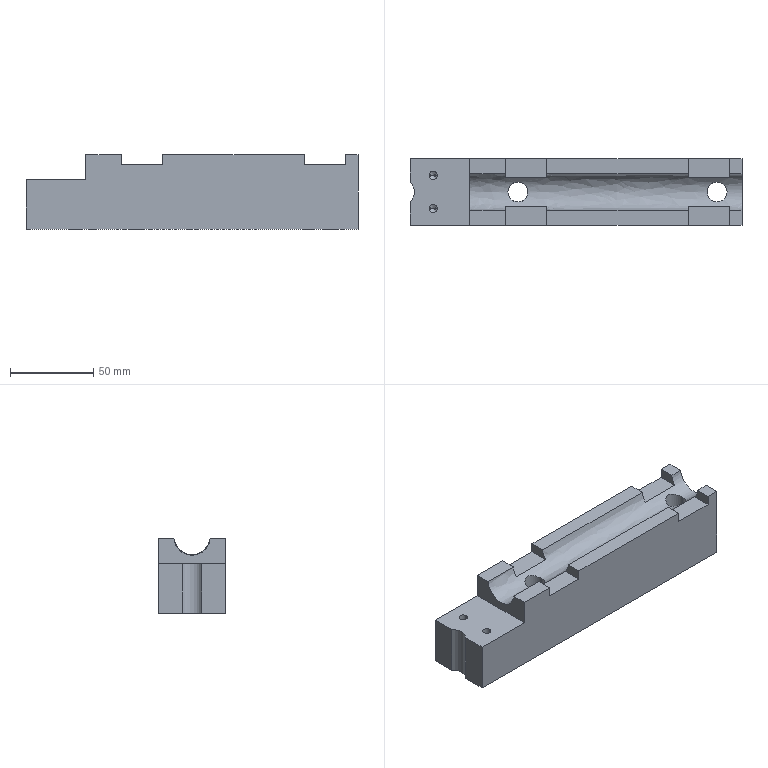NC program | NX | posted with a generic post
Lines 3384 to 4303 of 104568:
(FLOOR_WALL_1 , TOOL : D6)
N6760 T06 M6
N6762 G54
N6764 G17 G0 G90 X71.103 Y-24.5 S9500 M3
N6766 G43 Z30. H6
N6768 Z-4.5
N6770 G94 G1 Z-6. F1250.
N6772 Y-22.48
N6774 G3 X70.803 Y-23. R0.6
N6776 G1 Y-5.535
N6778 X73.431 Y-5.537
N6780 Y-23.
N6782 X76.059
N6784 Y-5.538
N6786 X78.687 Y-5.54
N6788 Y-23.
N6790 X81.316
N6792 Y-5.542
N6794 X83.944 Y-5.543
N6796 Y-23.
N6798 X86.572
N6800 Y-5.545
N6802 X89.2 Y-5.546
N6804 Y-23.
N6806 G2 X88.9 Y-23.52 R0.6
N6808 G1 X87.202 Y-24.5
N6810 Z-4.5
N6812 G0 Z30.
N6814 X87.502
N6816 Z-4.5
N6818 G1 Z-6.
N6820 X89.2 Y-23.52
N6822 G3 X89.5 Y-23. R0.6
N6824 G1 Y-5.546
N6826 G3 X89.2 Y-5.027 R0.6
N6828 G1 X87.5 Y-4.045
N6830 Z-4.5
N6832 G0 Z30.
N6834 X72.496 Y-4.036
N6836 Z-4.5
N6838 G1 Z-6.
N6840 X70.8 Y-5.015
N6842 G3 X70.5 Y-5.535 R0.6
N6844 G1 Y-23.
N6846 G3 X70.8 Y-23.52 R0.6
N6848 G1 X72.498 Y-24.5
N6850 Z-4.5
N6852 G0 Z30.
N6854 X71.101 Y3.926
N6856 Z-4.5
N6858 G1 Z-6.
N6860 X71.103 Y5.946
N6862 G3 X70.803 Y5.427 R0.6
N6864 G1 Y23.
N6866 X73.431
N6868 Y5.426
N6870 X76.059 Y5.425
N6872 Y23.
N6874 X78.687
N6876 Y5.425
N6878 X81.316 Y5.424
N6880 Y23.
N6882 X83.944
N6884 Y5.424
N6886 X86.572 Y5.423
N6888 Y23.
N6890 X89.2
N6892 Y5.422
N6894 G2 X88.9 Y4.902 R0.6
N6896 G1 X87.203 Y3.922
N6898 Z-4.5
N6900 G0 Z30.
N6902 X87.503
N6904 Z-4.5
N6906 G1 Z-6.
N6908 X89.2 Y4.902
N6910 G3 X89.5 Y5.422 R0.6
N6912 G1 Y23.
N6914 G3 X89.2 Y23.52 R0.6
N6916 G1 X87.502 Y24.5
N6918 Z-4.5
N6920 G0 Z30.
N6922 X72.498
N6924 Z-4.5
N6926 G1 Z-6.
N6928 X70.8 Y23.52
N6930 G3 X70.5 Y23. R0.6
N6932 G1 Y5.427
N6934 G3 X70.8 Y4.907 R0.6
N6936 G1 X72.499 Y3.926
N6938 Z-4.5
N6940 G0 Z30.
N6942 X-38.899 Y3.981
N6944 Z-4.5
N6946 G1 Z-6.
N6948 X-38.897 Y6.001
N6950 G3 X-39.197 Y5.481 R0.6
N6952 G1 Y23.
N6954 X-36.569
N6956 Y5.48
N6958 X-33.941
N6960 Y23.
N6962 X-31.313
N6964 Y5.479
N6966 X-28.684
N6968 Y23.
N6970 X-26.056
N6972 Y5.479
N6974 X-23.428
N6976 Y23.
N6978 X-20.8
N6980 Y5.479
N6982 G2 X-21.1 Y4.96 R0.6
N6984 G1 X-22.798 Y3.979
N6986 Z-4.5
N6988 G0 Z30.
N6990 X-22.498
N6992 Z-4.5
N6994 G1 Z-6.
N6996 X-20.8 Y4.96
N6998 G3 X-20.5 Y5.479 R0.6
N7000 G1 Y23.
N7002 G3 X-20.8 Y23.52 R0.6
N7004 G1 X-22.498 Y24.5
N7006 Z-4.5
N7008 G0 Z30.
N7010 X-37.502
N7012 Z-4.5
N7014 G1 Z-6.
N7016 X-39.2 Y23.52
N7018 G3 X-39.5 Y23. R0.6
N7020 G1 Y5.481
N7022 G3 X-39.2 Y4.962 R0.6
N7024 G1 X-37.499 Y3.98
N7026 Z-4.5
N7028 G0 Z30.
N7030 X-38.897 Y-24.5
N7032 Z-4.5
N7034 G1 Z-6.
N7036 Y-22.48
N7038 G3 X-39.197 Y-23. R0.6
N7040 G1 Y-5.482
N7042 X-36.569 Y-5.484
N7044 Y-23.
N7046 X-33.941
N7048 Y-5.485
N7050 X-31.313 Y-5.486
N7052 Y-23.
N7054 X-28.684
N7056 Y-5.488
N7058 X-26.056 Y-5.491
N7060 Y-23.
N7062 X-23.428
N7064 Y-5.493
N7066 X-20.8 Y-5.496
N7068 Y-23.
N7070 G2 X-21.1 Y-23.52 R0.6
N7072 G1 X-22.798 Y-24.5
N7074 Z-4.5
N7076 G0 Z30.
N7078 X-22.498
N7080 Z-4.5
N7082 G1 Z-6.
N7084 X-20.8 Y-23.52
N7086 G3 X-20.5 Y-23. R0.6
N7088 G1 Y-5.496
N7090 G3 X-20.8 Y-4.977 R0.6
N7092 G1 X-22.501 Y-3.994
N7094 Z-4.5
N7096 G0 Z30.
N7098 X-37.504 Y-3.983
N7100 Z-4.5
N7102 G1 Z-6.
N7104 X-39.2 Y-4.963
N7106 G3 X-39.5 Y-5.482 R0.6
N7108 G1 Y-23.
N7110 G3 X-39.2 Y-23.52 R0.6
N7112 G1 X-37.502 Y-24.5
N7114 Z-4.5
N7116 G0 Z30.
N7118 X-104.123 Y-23.995
N7120 Z-13.5
N7122 G1 Z-15.
N7124 X-103.3 Y-23.52
N7126 G3 X-103. Y-23. R0.6
N7128 G1 Y23.
N7130 X-100.025
N7132 Y-23.
N7134 X-97.05
N7136 Y23.
N7138 X-94.075
N7140 Y-23.
N7142 X-91.1
N7144 Y23.
N7146 X-88.125
N7148 Y-23.
N7150 X-85.15
N7152 Y23.
N7154 X-82.175
N7156 Y-23.
N7158 X-79.2
N7160 Y23.
N7162 X-76.225
N7164 Y-23.
N7166 X-73.25
N7168 Y23.
N7170 X-70.275
N7172 Y-23.
N7174 X-67.3
N7176 Y23.
N7178 G3 X-67.6 Y23.52 R0.6
N7180 G1 X-69.298 Y24.5
N7182 Z-13.5
N7184 G0 Z30.
N7186 X-68.998 Y-24.5
N7188 Z-13.5
N7190 G1 Z-15.
N7192 X-67.3 Y-23.52
N7194 G3 X-67. Y-23. R0.6
N7196 G1 Y23.
N7198 G3 X-67.3 Y23.52 R0.6
N7200 G1 X-68.998 Y24.5
N7202 Z-13.5
N7204 G0 Z30.
(FIXED_CONTOUR , TOOL : D6)
N7206 X-64.628 Y6.929
N7208 Z3.6
N7210 G1 Z-1.91 F500.
N7212 G2 X-64.472 Y7.508 R0.6
N7214 G1 X-64.378 Y7.602 Z-1.535 F2500.
N7216 X-64.225 Y7.755 Z-0.73
N7218 X-64.2 Y7.78 Z-0.573
N7220 X-64.091 Y7.889 Z0.362
N7222 X-63.94 Z0.366
N7224 X-64.047 Y7.781 Z-0.559
N7226 X-64.089 Y7.74 Z-0.823
N7228 X-64.21 Y7.619 Z-1.458
N7230 X-64.256 Y7.573 Z-1.656
N7232 X-64.414 Y7.415 Z-2.238
N7234 X-64.479 Y7.35 Z-2.423
N7236 X-64.488 Y7.159 Z-2.949
N7238 X-64.259 Y7.387 Z-2.324
N7240 X-64.215 Y7.431 Z-2.186
N7242 X-64.097 Y7.549 Z-1.749
N7244 X-64.007 Y7.639 Z-1.365
N7246 X-63.926 Y7.721 Z-0.934
N7248 X-63.864 Y7.783 Z-0.542
N7250 X-63.758 Y7.889 Z0.37
N7252 X-63.553 Z0.375
N7254 X-63.657 Y7.784 Z-0.523
N7256 X-63.742 Y7.7 Z-1.059
N7258 X-63.78 Y7.661 Z-1.26
N7260 X-63.919 Y7.523 Z-1.853
N7262 X-63.996 Y7.446 Z-2.139
N7264 X-64.085 Y7.356 Z-2.42
N7266 X-64.385 Y7.057 Z-3.23
N7268 X-64.493 Y6.948 Z-3.46
N7270 X-64.498 Y6.72 Z-3.942
N7272 X-64.161 Y7.057 Z-3.231
N7274 X-64.075 Y7.143 Z-3.01
N7276 X-63.896 Y7.322 Z-2.525
N7278 X-63.757 Y7.461 Z-2.088
N7280 X-63.724 Y7.494 Z-1.966
N7282 X-63.537 Y7.681 Z-1.169
N7284 X-63.433 Y7.785 Z-0.507
N7286 X-63.329 Y7.888 Z0.38
N7288 X-63.081 Z0.386
N7290 X-63.185 Y7.785 Z-0.491
N7292 X-63.289 Y7.681 Z-1.17
N7294 X-63.497 Y7.473 Z-2.051
N7296 X-63.686 Y7.284 Z-2.642
N7298 X-63.913 Y7.057 Z-3.232
N7300 X-64.33 Y6.64 Z-4.104
N7302 X-64.5 Y6.47 Z-4.396
N7304 X-64.501 Y6.209 Z-4.83
N7306 X-64.071 Y6.64 Z-4.104
N7308 X-63.654 Y7.057 Z-3.233
N7310 X-63.446 Y7.265 Z-2.701
N7312 X-63.238 Y7.473 Z-2.054
N7314 X-63.03 Y7.681 Z-1.172
N7316 X-62.926 Y7.785 Z-0.475
N7318 X-62.822 Y7.888 Z0.392
N7320 X-62.556 Z0.399
N7322 X-62.66 Y7.784 Z-0.465
N7324 X-62.764 Y7.681 Z-1.174
N7326 X-62.972 Y7.473 Z-2.056
N7328 X-63.18 Y7.265 Z-2.702
N7330 X-63.388 Y7.057 Z-3.234
N7332 X-63.804 Y6.64 Z-4.104
N7334 X-64.221 Y6.223 Z-4.81
N7336 X-64.5 Y5.944 Z-5.23
N7338 Y5.738 Z-5.522
N7340 Y5.655 Z-5.629
N7342 X-64.35 Y5.806 Z-5.43
N7344 X-63.933 Y6.223 Z-4.81
N7346 X-63.516 Y6.64 Z-4.104
N7348 X-63.099 Y7.057 Z-3.235
N7350 X-62.891 Y7.265 Z-2.703
N7352 X-62.683 Y7.473 Z-2.059
N7354 X-62.475 Y7.681 Z-1.174
N7356 X-62.371 Y7.784 Z-0.471
N7358 X-62.267 Y7.888 Z0.406
N7360 X-61.967 Z0.413
N7362 X-62.071 Y7.784 Z-0.478
N7364 X-62.175 Y7.681 Z-1.174
N7366 X-62.383 Y7.473 Z-2.059
N7368 X-62.591 Y7.265 Z-2.703
N7370 X-62.799 Y7.057 Z-3.235
N7372 X-63.215 Y6.64 Z-4.103
N7374 X-63.632 Y6.223 Z-4.81
N7376 X-64.049 Y5.806 Z-5.43
N7378 X-64.5 Y5.355 Z-6.009
N7380 Y5.054 Z-6.354
N7382 X-64.165 Y5.389 Z-5.971
N7384 X-63.748 Y5.806 Z-5.43
N7386 X-63.331 Y6.223 Z-4.81
N7388 X-62.914 Y6.64 Z-4.102
N7390 X-62.497 Y7.057 Z-3.236
N7392 X-62.289 Y7.265 Z-2.704
N7394 X-62.081 Y7.473 Z-2.06
N7396 X-61.873 Y7.681 Z-1.175
N7398 X-61.769 Y7.784 Z-0.485
N7400 X-61.665 Y7.889 Z0.419
N7402 X-61.364 Z0.424
N7404 X-61.468 Y7.784 Z-0.492
N7406 X-61.572 Y7.681 Z-1.172
N7408 X-61.78 Y7.473 Z-2.06
N7410 X-61.988 Y7.265 Z-2.705
N7412 X-62.196 Y7.057 Z-3.237
N7414 X-62.613 Y6.64 Z-4.101
N7416 X-63.03 Y6.223 Z-4.81
N7418 X-63.447 Y5.806 Z-5.429
N7420 X-63.864 Y5.389 Z-5.972
N7422 X-64.28 Y4.972 Z-6.443
N7424 X-64.5 Y4.753 Z-6.666
N7426 Y4.555 Z-6.862
N7428 Y4.451 Z-6.952
N7430 X-64.396 Y4.555 Z-6.862
N7432 X-63.979 Y4.972 Z-6.443
N7434 X-63.562 Y5.389 Z-5.972
N7436 X-63.145 Y5.806 Z-5.428
N7438 X-62.729 Y6.223 Z-4.809
N7440 X-62.312 Y6.64 Z-4.1
N7442 X-61.895 Y7.057 Z-3.237
N7444 X-61.687 Y7.265 Z-2.706
N7446 X-61.479 Y7.473 Z-2.06
N7448 X-61.271 Y7.681 Z-1.169
N7450 X-61.167 Y7.784 Z-0.499
N7452 X-61.063 Y7.889 Z0.43
N7454 X-60.761 Z0.435
N7456 X-60.866 Y7.784 Z-0.504
N7458 X-60.97 Y7.681 Z-1.167
N7460 X-61.178 Y7.473 Z-2.061
N7462 X-61.386 Y7.265 Z-2.706
N7464 X-61.593 Y7.057 Z-3.238
N7466 X-62.01 Y6.64 Z-4.099
N7468 X-62.427 Y6.223 Z-4.809
N7470 X-62.844 Y5.806 Z-5.427
N7472 X-63.261 Y5.389 Z-5.972
N7474 X-63.678 Y4.972 Z-6.443
N7476 X-64.095 Y4.555 Z-6.862
N7478 X-64.5 Y4.15 Z-7.214
N7480 X-64.501 Y3.848 Z-7.475
N7482 X-63.793 Y4.555 Z-6.862
N7484 X-63.377 Y4.972 Z-6.444
N7486 X-62.96 Y5.389 Z-5.971
N7488 X-62.543 Y5.806 Z-5.427
N7490 X-62.126 Y6.223 Z-4.808
N7492 X-61.709 Y6.64 Z-4.099
N7494 X-61.292 Y7.057 Z-3.238
N7496 X-61.084 Y7.265 Z-2.707
N7498 X-60.876 Y7.473 Z-2.061
N7500 X-60.668 Y7.681 Z-1.166
N7502 X-60.564 Y7.784 Z-0.509
N7504 X-60.46 Y7.889 Z0.44
N7506 X-60.159 Z0.445
N7508 X-60.263 Y7.784 Z-0.513
N7510 X-60.367 Y7.681 Z-1.164
N7512 X-60.575 Y7.473 Z-2.061
N7514 X-60.783 Y7.265 Z-2.708
N7516 X-60.991 Y7.057 Z-3.238
N7518 X-61.408 Y6.64 Z-4.098
N7520 X-61.824 Y6.223 Z-4.807
N7522 X-62.241 Y5.806 Z-5.426
N7524 X-62.658 Y5.389 Z-5.971
N7526 X-63.075 Y4.972 Z-6.444
N7528 X-63.492 Y4.555 Z-6.863
N7530 X-64.326 Y3.722 Z-7.586
N7532 X-64.501 Y3.547 Z-7.71
N7534 Y3.247 Z-7.923
N7536 X-64.026 Y3.722 Z-7.586
N7538 X-63.192 Y4.555 Z-6.862
N7540 X-62.775 Y4.972 Z-6.444
N7542 X-62.358 Y5.389 Z-5.97
N7544 X-61.941 Y5.806 Z-5.425
N7546 X-61.524 Y6.223 Z-4.805
N7548 X-61.107 Y6.64 Z-4.097
N7550 X-60.691 Y7.057 Z-3.236
N7552 X-60.483 Y7.265 Z-2.708
N7554 X-60.275 Y7.473 Z-2.062
N7556 X-60.067 Y7.68 Z-1.165
N7558 X-59.963 Y7.784 Z-0.515
N7560 X-59.859 Y7.889 Z0.449
N7562 X-59.557 Y7.888 Z0.452
N7564 X-59.661 Y7.784 Z-0.517
N7566 X-59.765 Y7.68 Z-1.17
N7568 X-59.973 Y7.473 Z-2.063
N7570 X-60.181 Y7.265 Z-2.709
N7572 X-60.389 Y7.057 Z-3.235
N7574 X-60.806 Y6.64 Z-4.095
N7576 X-61.223 Y6.223 Z-4.803
N7578 X-61.64 Y5.806 Z-5.424
N7580 X-62.056 Y5.389 Z-5.969
N7582 X-62.473 Y4.972 Z-6.444
N7584 X-62.89 Y4.555 Z-6.862
N7586 X-63.724 Y3.722 Z-7.586
N7588 X-64.501 Y2.945 Z-8.137
N7590 Y2.888 Z-8.178
N7592 Y2.643 Z-8.321
N7594 X-64.256 Y2.888 Z-8.178
N7596 X-63.422 Y3.722 Z-7.586
N7598 X-62.589 Y4.555 Z-6.861
N7600 X-62.172 Y4.972 Z-6.443
N7602 X-61.755 Y5.389 Z-5.968
N7604 X-61.338 Y5.806 Z-5.423
N7606 X-60.921 Y6.223 Z-4.801
N7608 X-60.504 Y6.64 Z-4.094
N7610 X-60.087 Y7.057 Z-3.233
N7612 X-59.879 Y7.265 Z-2.709
N7614 X-59.671 Y7.472 Z-2.064
N7616 X-59.464 Y7.68 Z-1.174
N7618 X-59.36 Y7.784 Z-0.518
N7620 X-59.256 Y7.888 Z0.455
N7622 X-58.954 Z0.458
N7624 X-59.058 Y7.784 Z-0.52
N7626 X-59.162 Y7.68 Z-1.177
N7628 X-59.37 Y7.472 Z-2.066
N7630 X-59.578 Y7.265 Z-2.71
N7632 X-59.785 Y7.057 Z-3.232
N7634 X-60.202 Y6.64 Z-4.093
N7636 X-60.619 Y6.223 Z-4.8
N7638 X-61.036 Y5.806 Z-5.422
N7640 X-61.453 Y5.389 Z-5.967
N7642 X-61.87 Y4.972 Z-6.443
N7644 X-62.287 Y4.555 Z-6.857
N7646 X-63.121 Y3.722 Z-7.586
N7648 X-63.954 Y2.888 Z-8.179
N7650 X-64.501 Y2.341 Z-8.497
N7652 Y2.04 Z-8.672
N7654 X-63.653 Y2.888 Z-8.179
N7656 X-62.819 Y3.722 Z-7.585
N7658 X-61.985 Y4.555 Z-6.854
N7660 X-61.568 Y4.972 Z-6.442
N7662 X-61.151 Y5.389 Z-5.967
N7664 X-60.734 Y5.806 Z-5.422
N7666 X-60.318 Y6.223 Z-4.8
N7668 X-59.901 Y6.64 Z-4.094
N7670 X-59.484 Y7.057 Z-3.23
N7672 X-59.276 Y7.265 Z-2.71
N7674 X-59.068 Y7.472 Z-2.068
N7676 X-58.861 Y7.68 Z-1.179
N7678 X-58.757 Y7.784 Z-0.522
N7680 X-58.653 Y7.888 Z0.461
N7682 X-58.351 Y7.887 Z0.464
N7684 X-58.455 Y7.783 Z-0.523
N7686 X-58.559 Y7.68 Z-1.181
N7688 X-58.767 Y7.472 Z-2.07
N7690 X-58.974 Y7.264 Z-2.711
N7692 X-59.182 Y7.057 Z-3.228
N7694 X-59.599 Y6.64 Z-4.095
N7696 X-60.016 Y6.223 Z-4.8
N7698 X-60.433 Y5.806 Z-5.422
N7700 X-60.85 Y5.389 Z-5.966
N7702 X-61.266 Y4.972 Z-6.442
N7704 X-61.683 Y4.555 Z-6.852
N7706 X-62.517 Y3.722 Z-7.585
N7708 X-63.351 Y2.888 Z-8.179
N7710 X-64.185 Y2.054 Z-8.666
N7712 X-64.501 Y1.738 Z-8.814
N7714 Y1.436 Z-8.955
N7716 X-63.883 Y2.054 Z-8.666
N7718 X-63.049 Y2.888 Z-8.179
N7720 X-62.215 Y3.722 Z-7.585
N7722 X-61.382 Y4.555 Z-6.852
N7724 X-60.965 Y4.972 Z-6.441
N7726 X-60.548 Y5.389 Z-5.966
N7728 X-60.131 Y5.806 Z-5.422
N7730 X-59.714 Y6.223 Z-4.801
N7732 X-59.297 Y6.64 Z-4.096
N7734 X-58.88 Y7.057 Z-3.226
N7736 X-58.673 Y7.264 Z-2.711
N7738 X-58.465 Y7.472 Z-2.071
N7740 X-58.257 Y7.68 Z-1.181
N7742 X-58.154 Y7.783 Z-0.522
N7744 X-58.05 Y7.887 Z0.467
N7746 X-57.748 Z0.47
N7748 X-57.852 Y7.783 Z-0.522
N7750 X-57.956 Y7.68 Z-1.181
N7752 X-58.163 Y7.472 Z-2.072
N7754 X-58.371 Y7.264 Z-2.712
N7756 X-58.579 Y7.057 Z-3.223
N7758 X-58.996 Y6.64 Z-4.096
N7760 X-59.412 Y6.223 Z-4.802
N7762 X-59.829 Y5.806 Z-5.423
N7764 X-60.246 Y5.389 Z-5.966
N7766 X-60.663 Y4.972 Z-6.441
N7768 X-61.08 Y4.555 Z-6.851
N7770 X-61.914 Y3.722 Z-7.585
N7772 X-62.748 Y2.888 Z-8.179
N7774 X-63.58 Y2.055 Z-8.665
N7776 X-64.415 Y1.22 Z-9.057
N7778 X-64.501 Y1.134 Z-9.088
N7780 Y0.833 Z-9.199
N7782 X-64.113 Y1.22 Z-9.057
N7784 X-63.28 Y2.054 Z-8.666
N7786 X-62.446 Y2.888 Z-8.179
N7788 X-61.612 Y3.722 Z-7.584
N7790 X-60.778 Y4.555 Z-6.852
N7792 X-60.361 Y4.972 Z-6.441
N7794 X-59.945 Y5.389 Z-5.966
N7796 X-59.528 Y5.806 Z-5.424
N7798 X-59.111 Y6.223 Z-4.803
N7800 X-58.694 Y6.64 Z-4.096
N7802 X-58.277 Y7.057 Z-3.221
N7804 X-58.069 Y7.264 Z-2.712
N7806 X-57.862 Y7.472 Z-2.072
N7808 X-57.654 Y7.68 Z-1.181
N7810 X-57.55 Y7.784 Z-0.521
N7812 X-57.446 Y7.888 Z0.473
N7814 X-57.144 Z0.474
N7816 X-57.249 Y7.784 Z-0.518
N7818 X-57.353 Y7.68 Z-1.18
N7820 X-57.56 Y7.472 Z-2.072
N7822 X-57.768 Y7.264 Z-2.712
N7824 X-57.976 Y7.057 Z-3.218
N7826 X-58.393 Y6.64 Z-4.095
N7828 X-58.809 Y6.223 Z-4.803
N7830 X-59.226 Y5.806 Z-5.425
N7832 X-59.643 Y5.389 Z-5.967
N7834 X-60.06 Y4.972 Z-6.441
N7836 X-60.477 Y4.555 Z-6.852
N7838 X-61.311 Y3.722 Z-7.584
N7840 X-62.145 Y2.888 Z-8.179
N7842 X-62.978 Y2.054 Z-8.665
N7844 X-63.812 Y1.22 Z-9.057
N7846 X-64.501 Y0.532 Z-9.311
N7848 Y0.352 Z-9.375
N7850 Y0.232 Z-9.413
N7852 X-64.346 Y0.387 Z-9.364
N7854 X-63.512 Y1.22 Z-9.058
N7856 X-62.679 Y2.054 Z-8.665
N7858 X-61.845 Y2.888 Z-8.179
N7860 X-61.011 Y3.722 Z-7.584
N7862 X-60.177 Y4.555 Z-6.853
N7864 X-59.76 Y4.972 Z-6.441
N7866 X-59.344 Y5.389 Z-5.967
N7868 X-58.927 Y5.806 Z-5.426
N7870 X-58.508 Y6.225 Z-4.801
N7872 X-58.093 Y6.64 Z-4.094
N7874 X-57.676 Y7.057 Z-3.216
N7876 X-57.468 Y7.264 Z-2.711
N7878 X-57.261 Y7.472 Z-2.071
N7880 X-57.053 Y7.68 Z-1.179
N7882 X-56.949 Y7.784 Z-0.516
N7884 X-56.844 Y7.888 Z0.475
N7886 X-56.544 Y7.889 Z0.477
N7888 X-56.649 Y7.784 Z-0.513
N7890 X-56.753 Y7.68 Z-1.178
N7892 X-56.961 Y7.472 Z-2.07
N7894 X-57.169 Y7.264 Z-2.71
N7896 X-57.376 Y7.057 Z-3.213
N7898 X-57.793 Y6.64 Z-4.093
N7900 X-58.21 Y6.223 Z-4.805
N7902 X-58.627 Y5.806 Z-5.427
N7904 X-59.044 Y5.389 Z-5.968
N7906 X-59.461 Y4.972 Z-6.441
N7908 X-59.878 Y4.555 Z-6.853
N7910 X-60.711 Y3.722 Z-7.583
N7912 X-61.545 Y2.888 Z-8.179
N7914 X-62.379 Y2.054 Z-8.665
N7916 X-63.213 Y1.22 Z-9.058
N7918 X-64.046 Y0.387 Z-9.365
N7920 X-64.432 Y0.001 Z-9.483
N7922 X-64.5 Y-0.067 Z-9.463
N7924 Y-0.368 Z-9.368
N7926 X-64.131 Y0.001 Z-9.483
N7928 X-63.745 Y0.387 Z-9.365
N7930 X-62.911 Y1.22 Z-9.058
N7932 X-62.077 Y2.054 Z-8.664
N7934 X-61.244 Y2.888 Z-8.179
N7936 X-60.41 Y3.722 Z-7.583
N7938 X-59.576 Y4.555 Z-6.854
N7940 X-59.159 Y4.972 Z-6.442
N7942 X-58.742 Y5.389 Z-5.968
N7944 X-58.325 Y5.806 Z-5.427
N7946 X-57.909 Y6.223 Z-4.806
N7948 X-57.492 Y6.64 Z-4.091
N7950 X-57.075 Y7.057 Z-3.211
N7952 X-56.867 Y7.265 Z-2.709
N7954 X-56.659 Y7.472 Z-2.068
N7956 X-56.451 Y7.681 Z-1.176
N7958 X-56.347 Y7.785 Z-0.509
N7960 X-56.243 Y7.889 Z0.478
N7962 X-55.943 Z0.479
N7964 X-56.047 Y7.785 Z-0.506
N7966 X-56.151 Y7.681 Z-1.174
N7968 X-56.359 Y7.473 Z-2.067
N7970 X-56.567 Y7.265 Z-2.707
N7972 X-56.775 Y7.057 Z-3.208
N7974 X-57.192 Y6.64 Z-4.09
N7976 X-57.609 Y6.223 Z-4.807
N7978 X-58.026 Y5.806 Z-5.428
N7980 X-58.443 Y5.389 Z-5.969
N7982 X-58.86 Y4.972 Z-6.442
N7984 X-59.276 Y4.555 Z-6.854
N7986 X-60.11 Y3.722 Z-7.583
N7988 X-60.944 Y2.888 Z-8.178
N7990 X-61.778 Y2.054 Z-8.664
N7992 X-62.612 Y1.22 Z-9.057
N7994 X-63.445 Y0.387 Z-9.365
N7996 X-63.831 Y0.001 Z-9.483
N7998 X-64.279 Y-0.447 Z-9.343
N8000 X-64.5 Y-0.668 Z-9.258
N8002 Y-0.968 Z-9.143
N8004 X-63.979 Y-0.447 Z-9.343
N8006 X-63.532 Y0.001 Z-9.483
N8008 X-63.146 Y0.387 Z-9.365
N8010 X-62.312 Y1.22 Z-9.057
N8012 X-61.478 Y2.054 Z-8.664
N8014 X-60.644 Y2.888 Z-8.178
N8016 X-59.811 Y3.722 Z-7.582
N8018 X-58.977 Y4.555 Z-6.855
N8020 X-58.56 Y4.972 Z-6.442
N8022 X-58.143 Y5.389 Z-5.969
N8024 X-57.726 Y5.806 Z-5.429
N8026 X-57.309 Y6.223 Z-4.808
N8028 X-56.892 Y6.64 Z-4.089
N8030 X-56.475 Y7.057 Z-3.206
N8032 X-56.267 Y7.265 Z-2.706
N8034 X-56.059 Y7.473 Z-2.065
N8036 X-55.851 Y7.681 Z-1.173
N8038 X-55.747 Y7.785 Z-0.505
N8040 X-55.643 Y7.89 Z0.481
N8042 X-55.343 Z0.482
N8044 X-55.447 Y7.785 Z-0.505
N8046 X-55.552 Y7.681 Z-1.174
N8048 X-55.76 Y7.473 Z-2.064
N8050 X-55.968 Y7.265 Z-2.704
N8052 X-56.176 Y7.057 Z-3.203
N8054 X-56.593 Y6.64 Z-4.087
N8056 X-57.01 Y6.223 Z-4.809
N8058 X-57.426 Y5.806 Z-5.43
N8060 X-57.843 Y5.389 Z-5.97
N8062 X-58.26 Y4.972 Z-6.442
N8064 X-58.677 Y4.555 Z-6.855
N8066 X-59.511 Y3.722 Z-7.582
N8068 X-60.345 Y2.888 Z-8.177
N8070 X-61.178 Y2.054 Z-8.663
N8072 X-62.012 Y1.22 Z-9.057
N8074 X-62.846 Y0.387 Z-9.365
N8076 X-63.232 Y0. Z-9.483
N8078 X-63.68 Y-0.447 Z-9.344
N8080 X-64.5 Y-1.267 Z-9.029
N8082 Y-1.567 Z-8.887
N8084 X-64.214 Y-1.281 Z-9.024
N8086 X-63.38 Y-0.447 Z-9.344
N8088 X-62.933 Y0. Z-9.483
N8090 X-62.546 Y0.387 Z-9.365
N8092 X-61.713 Y1.22 Z-9.057
N8094 X-60.879 Y2.054 Z-8.663
N8096 X-60.045 Y2.888 Z-8.177
N8098 X-59.211 Y3.722 Z-7.582
N8100 X-58.377 Y4.555 Z-6.855
N8102 X-57.961 Y4.972 Z-6.442
N8104 X-57.544 Y5.389 Z-5.97
N8106 X-57.127 Y5.806 Z-5.431
N8108 X-56.71 Y6.223 Z-4.809
N8110 X-56.293 Y6.64 Z-4.086
N8112 X-55.876 Y7.057 Z-3.201
N8114 X-55.668 Y7.265 Z-2.703
N8116 X-55.46 Y7.473 Z-2.064
N8118 X-55.252 Y7.681 Z-1.174
N8120 X-55.148 Y7.785 Z-0.506
N8122 X-55.043 Y7.89 Z0.483
N8124 X-54.743 Y7.891 Z0.484
N8126 X-54.848 Y7.785 Z-0.503
N8128 X-54.952 Y7.681 Z-1.175
N8130 X-55.16 Y7.473 Z-2.063
N8132 X-55.368 Y7.265 Z-2.702
N8134 X-55.576 Y7.057 Z-3.199
N8136 X-55.993 Y6.64 Z-4.085
N8138 X-56.41 Y6.223 Z-4.81
N8140 X-56.827 Y5.806 Z-5.432
N8142 X-57.244 Y5.389 Z-5.97
N8144 X-57.659 Y4.974 Z-6.44
N8146 X-58.078 Y4.555 Z-6.854
N8148 X-58.912 Y3.722 Z-7.581
N8150 X-59.745 Y2.888 Z-8.177
N8152 X-60.579 Y2.054 Z-8.663
N8154 X-61.413 Y1.22 Z-9.056
N8156 X-62.247 Y0.387 Z-9.365
N8158 X-62.633 Y0. Z-9.483
N8160 X-63.08 Y-0.447 Z-9.344
N8162 X-63.914 Y-1.281 Z-9.024
N8164 X-64.5 Y-1.867 Z-8.744
N8166 Y-2.129 Z-8.618
N8168 Y-2.166 Z-8.596
N8170 X-64.448 Y-2.115 Z-8.626
N8172 X-63.615 Y-1.281 Z-9.024
N8174 X-62.781 Y-0.447 Z-9.344
N8176 X-62.333 Y0. Z-9.483
N8178 X-61.947 Y0.387 Z-9.365
N8180 X-61.113 Y1.22 Z-9.056
N8182 X-60.279 Y2.054 Z-8.662
N8184 X-59.446 Y2.888 Z-8.176
N8186 X-58.612 Y3.722 Z-7.581
N8188 X-57.778 Y4.555 Z-6.853
N8190 X-57.361 Y4.972 Z-6.442
N8192 X-56.944 Y5.389 Z-5.971
N8194 X-56.527 Y5.806 Z-5.433
N8196 X-56.111 Y6.223 Z-4.811
N8198 X-55.694 Y6.64 Z-4.084
N8200 X-55.277 Y7.057 Z-3.197
N8202 X-55.069 Y7.265 Z-2.701
N8204 X-54.86 Y7.473 Z-2.063
N8206 X-54.652 Y7.682 Z-1.176
N8208 X-54.548 Y7.786 Z-0.5
N8210 X-54.443 Y7.891 Z0.486
N8212 X-54.143 Z0.487
N8214 X-54.248 Y7.786 Z-0.498
N8216 X-54.352 Y7.682 Z-1.177
N8218 X-54.561 Y7.473 Z-2.063
N8220 X-54.769 Y7.265 Z-2.701
N8222 X-54.977 Y7.057 Z-3.197
N8224 X-55.394 Y6.64 Z-4.083
N8226 X-55.811 Y6.223 Z-4.812
N8228 X-56.228 Y5.806 Z-5.433
N8230 X-56.645 Y5.389 Z-5.971
N8232 X-57.062 Y4.972 Z-6.443
N8234 X-57.539 Y4.495 Z-6.91
N8236 X-58.312 Y3.722 Z-7.58
N8238 X-59.146 Y2.888 Z-8.176
N8240 X-59.98 Y2.054 Z-8.662
N8242 X-60.814 Y1.22 Z-9.056
N8244 X-61.647 Y0.387 Z-9.365
N8246 X-62.033 Y0. Z-9.483
N8248 X-62.481 Y-0.447 Z-9.344
N8250 X-63.315 Y-1.281 Z-9.023
N8252 X-64.149 Y-2.115 Z-8.627
N8254 X-64.5 Y-2.466 Z-8.418
N8256 Y-2.766 Z-8.24
N8258 X-63.849 Y-2.115 Z-8.627
N8260 X-63.015 Y-1.281 Z-9.023
N8262 X-62.181 Y-0.447 Z-9.344
N8264 X-61.734 Y0.001 Z-9.483
N8266 X-61.348 Y0.387 Z-9.365
N8268 X-60.514 Y1.22 Z-9.055
N8270 X-59.68 Y2.054 Z-8.662
N8272 X-58.846 Y2.888 Z-8.175
N8274 X-58.013 Y3.722 Z-7.58
N8276 X-57.663 Y4.072 Z-7.274
N8278 X-57.339 Y4.396 Z-7.003
N8280 X-56.762 Y4.972 Z-6.443
N8282 X-56.345 Y5.389 Z-5.971
N8284 X-55.928 Y5.806 Z-5.434
N8286 X-55.511 Y6.223 Z-4.812
N8288 X-55.094 Y6.64 Z-4.082
N8290 X-54.678 Y7.057 Z-3.198
N8292 X-54.469 Y7.265 Z-2.7
N8294 X-54.261 Y7.474 Z-2.062
N8296 X-54.052 Y7.682 Z-1.179
N8298 X-53.948 Y7.786 Z-0.506
N8300 X-53.843 Y7.892 Z0.488
N8302 X-53.543 Z0.49
N8304 X-53.648 Y7.786 Z-0.514
N8306 X-53.753 Y7.682 Z-1.182
N8308 X-53.961 Y7.474 Z-2.063
N8310 X-54.169 Y7.265 Z-2.7
N8312 X-54.378 Y7.057 Z-3.2
N8314 X-54.795 Y6.64 Z-4.084
N8316 X-55.212 Y6.223 Z-4.813
N8318 X-55.629 Y5.806 Z-5.434
N8320 X-56.045 Y5.389 Z-5.971
N8322 X-56.462 Y4.972 Z-6.443
N8324 X-56.879 Y4.555 Z-6.851
N8326 X-57.138 Y4.297 Z-7.096
N8328 X-57.713 Y3.722 Z-7.58
N8330 X-58.547 Y2.888 Z-8.175
N8332 X-59.38 Y2.054 Z-8.661
N8334 X-60.214 Y1.22 Z-9.055
N8336 X-61.044 Y0.39 Z-9.363
N8338 X-61.434 Y0.001 Z-9.483
N8340 X-61.882 Y-0.447 Z-9.344
N8342 X-62.716 Y-1.281 Z-9.023
N8344 X-63.549 Y-2.115 Z-8.627
N8346 X-64.383 Y-2.949 Z-8.132
N8348 X-64.5 Y-3.066 Z-8.048
N8350 Y-3.366 Z-7.831
N8352 X-64.082 Y-2.949 Z-8.133
N8354 X-63.249 Y-2.115 Z-8.627
N8356 X-62.415 Y-1.281 Z-9.022
N8358 X-61.581 Y-0.447 Z-9.343
N8360 X-61.133 Y0. Z-9.483
N8362 X-60.747 Y0.387 Z-9.365
N8364 X-59.913 Y1.22 Z-9.055
N8366 X-59.08 Y2.054 Z-8.661
N8368 X-58.246 Y2.888 Z-8.174
N8370 X-57.412 Y3.722 Z-7.579
N8372 X-57.168 Y3.965 Z-7.384
N8374 X-56.936 Y4.197 Z-7.19
N8376 X-56.378 Y4.756 Z-6.654
N8378 X-56.161 Y4.972 Z-6.443
N8380 X-55.745 Y5.389 Z-5.971
N8382 X-55.328 Y5.806 Z-5.434
N8384 X-54.911 Y6.223 Z-4.813
N8386 X-54.494 Y6.64 Z-4.085
N8388 X-54.077 Y7.057 Z-3.201
N8390 X-53.869 Y7.265 Z-2.699
N8392 X-53.66 Y7.474 Z-2.063
N8394 X-53.452 Y7.682 Z-1.185
N8396 X-53.348 Y7.786 Z-0.522
N8398 X-53.241 Y7.892 Z0.49
N8400 X-52.941
N8402 X-53.048 Y7.786 Z-0.53
N8404 X-53.152 Y7.682 Z-1.188
N8406 X-53.36 Y7.474 Z-2.064
N8408 X-53.569 Y7.265 Z-2.699
N8410 X-53.777 Y7.057 Z-3.202
N8412 X-54.194 Y6.64 Z-4.086
N8414 X-54.611 Y6.223 Z-4.812
N8416 X-55.028 Y5.806 Z-5.434
N8418 X-55.445 Y5.389 Z-5.971
N8420 X-55.862 Y4.972 Z-6.442
N8422 X-56.456 Y4.377 Z-7.02
N8424 X-56.695 Y4.139 Z-7.245
N8426 X-57.112 Y3.722 Z-7.579
N8428 X-57.946 Y2.888 Z-8.174
N8430 X-58.78 Y2.054 Z-8.66
N8432 X-59.613 Y1.22 Z-9.054
N8434 X-60.447 Y0.387 Z-9.365
N8436 X-60.833 Y0. Z-9.483
N8438 X-61.281 Y-0.447 Z-9.343
N8440 X-62.115 Y-1.281 Z-9.022
N8442 X-62.949 Y-2.115 Z-8.627
N8444 X-63.782 Y-2.949 Z-8.133
N8446 X-64.5 Y-3.666 Z-7.615
N8448 Y-3.806 Z-7.511
N8450 Y-3.966 Z-7.369
N8452 X-64.316 Y-3.782 Z-7.531
N8454 X-63.483 Y-2.949 Z-8.133
N8456 X-62.649 Y-2.115 Z-8.627
N8458 X-61.815 Y-1.281 Z-9.021
N8460 X-60.981 Y-0.447 Z-9.343
N8462 X-60.534 Y0. Z-9.483
N8464 X-60.147 Y0.387 Z-9.365
N8466 X-59.314 Y1.22 Z-9.054
N8468 X-58.48 Y2.054 Z-8.66
N8470 X-57.646 Y2.888 Z-8.174
N8472 X-56.812 Y3.722 Z-7.578
N8474 X-56.396 Y4.139 Z-7.246
N8476 X-55.972 Y4.562 Z-6.842
N8478 X-55.562 Y4.972 Z-6.442
N8480 X-55.145 Y5.389 Z-5.97
N8482 X-54.728 Y5.806 Z-5.435
N8484 X-54.311 Y6.223 Z-4.812
N8486 X-53.894 Y6.64 Z-4.086
N8488 X-53.477 Y7.057 Z-3.203
N8490 X-53.269 Y7.265 Z-2.698
N8492 X-53.06 Y7.474 Z-2.064
N8494 X-52.852 Y7.682 Z-1.191
N8496 X-52.748 Y7.786 Z-0.538
N8498 X-52.641 Y7.893 Z0.489
N8500 X-52.341 Z0.488
N8502 X-52.448 Y7.786 Z-0.546
N8504 X-52.552 Y7.682 Z-1.194
N8506 X-52.761 Y7.474 Z-2.063
N8508 X-52.969 Y7.265 Z-2.697
N8510 X-53.178 Y7.057 Z-3.205
N8512 X-53.594 Y6.64 Z-4.085
N8514 X-54.011 Y6.223 Z-4.812
N8516 X-54.428 Y5.806 Z-5.437
N8518 X-54.845 Y5.389 Z-5.97
N8520 X-55.262 Y4.972 Z-6.442
N8522 X-55.972 Y4.262 Z-7.128
N8524 X-56.096 Y4.139 Z-7.246
N8526 X-56.513 Y3.722 Z-7.578
N8528 X-57.346 Y2.888 Z-8.173
N8530 X-58.18 Y2.054 Z-8.66
N8532 X-59.014 Y1.22 Z-9.054
N8534 X-59.848 Y0.387 Z-9.365
N8536 X-60.234 Y0. Z-9.483
N8538 X-60.682 Y-0.447 Z-9.343
N8540 X-61.515 Y-1.281 Z-9.021
N8542 X-62.349 Y-2.115 Z-8.626
N8544 X-63.183 Y-2.949 Z-8.132
N8546 X-64.017 Y-3.782 Z-7.532
N8548 X-64.499 Y-4.265 Z-7.105
N8550 Y-4.564 Z-6.842
N8552 X-63.717 Y-3.782 Z-7.532
N8554 X-62.883 Y-2.949 Z-8.132
N8556 X-62.049 Y-2.115 Z-8.626
N8558 X-61.216 Y-1.281 Z-9.021
N8560 X-60.382 Y-0.447 Z-9.343
N8562 X-59.934 Y0. Z-9.483
N8564 X-59.548 Y0.387 Z-9.365
N8566 X-58.714 Y1.22 Z-9.053
N8568 X-57.88 Y2.054 Z-8.659
N8570 X-57.047 Y2.888 Z-8.173
N8572 X-56.213 Y3.722 Z-7.577
N8574 X-55.796 Y4.139 Z-7.247
N8576 X-54.962 Y4.972 Z-6.442
N8578 X-54.545 Y5.389 Z-5.97
N8580 X-54.128 Y5.806 Z-5.437
N8582 X-53.712 Y6.223 Z-4.811
N8584 X-53.295 Y6.64 Z-4.084
N8586 X-52.878 Y7.057 Z-3.206